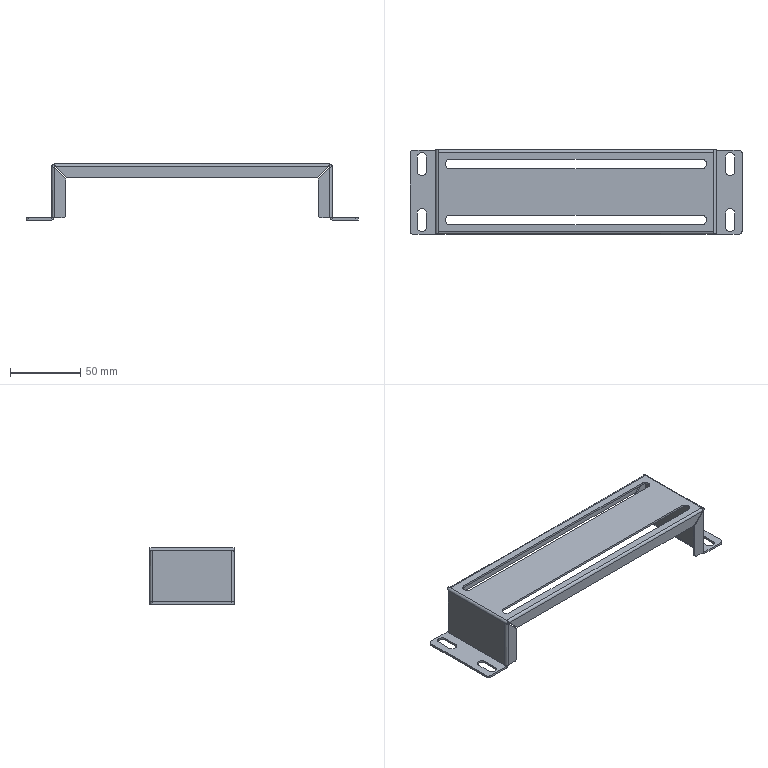Part | STEP file | FBDS-BJ-012 | 1 solid | 132 faces | box 237 x 60 x 40 mm | volume 29907 mm3 | plane 82 | cylinder 42 | spline 8 | commonest cylinder face diameters 0.4 x10 3.4 x10 4 x8 6.5 x8 6.6 x6